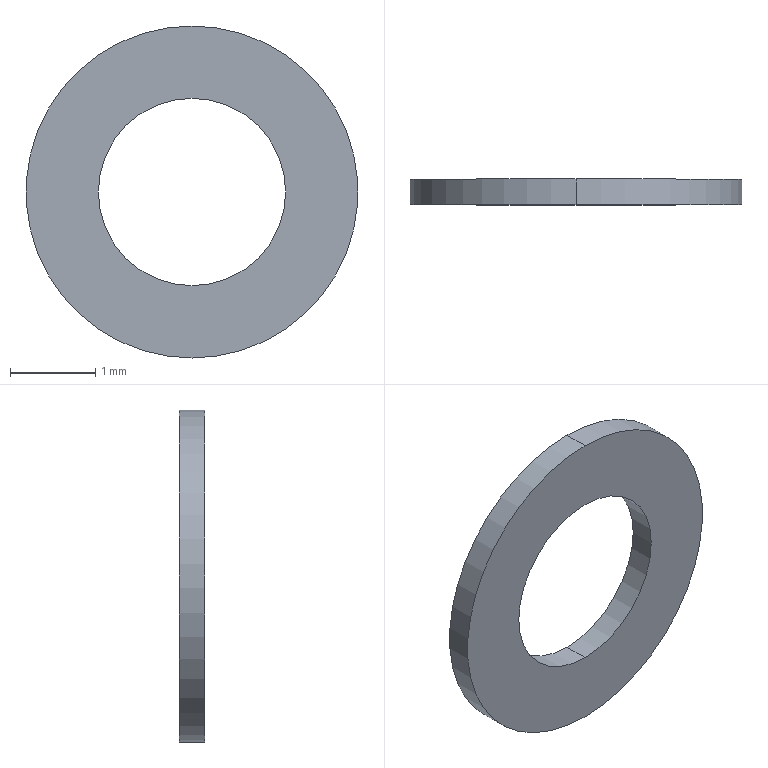Part | STEP file | _1-SO-126050001_1_1_1 | 1 solid | 6 faces | box 3.9 x 0.3 x 3.9 mm | volume 2.443 mm3 | cylinder 4 | plane 2 | commonest cylinder face diameters 2.2 x2 3.9 x2
STEP:
#1=CARTESIAN_POINT('',(0.,0.,0.));
#2=DIRECTION('',(0.,0.,1.));
#3=DIRECTION('',(1.,0.,0.));
#4=AXIS2_PLACEMENT_3D('',#1,#2,#3);
#5=CARTESIAN_POINT('',(-1.5,40.6,-81.15));
#6=VERTEX_POINT('',#5);
#7=CARTESIAN_POINT('',(-1.5,40.9,-81.15));
#8=VERTEX_POINT('',#7);
#9=CARTESIAN_POINT('',(-1.5,40.6,-81.15));
#10=DIRECTION('',(0.,1.,0.));
#11=VECTOR('',#10,1.);
#12=LINE('',#9,#11);
#13=CARTESIAN_POINT('',(-1.5,40.6,-82.25));
#14=DIRECTION('',(0.,1.,0.));
#15=DIRECTION('',(0.,0.,1.));
#16=AXIS2_PLACEMENT_3D('',#13,#14,#15);
#17=CYLINDRICAL_SURFACE('',#16,1.1);
#18=CARTESIAN_POINT('',(6.283,0.));
#19=DIRECTION('',(0.,1.));
#20=VECTOR('',#19,1.);
#21=LINE('',#18,#20);
#22=(GEOMETRIC_REPRESENTATION_CONTEXT(2)PARAMETRIC_REPRESENTATION_CONTEXT()REPRESENTATION_CONTEXT('',''));
#23=DEFINITIONAL_REPRESENTATION('',(#21),#22);
#24=PCURVE('',#17,#23);
#25=CARTESIAN_POINT('',(-1.5,40.6,-82.25));
#26=DIRECTION('',(0.,1.,0.));
#27=DIRECTION('',(0.,0.,1.));
#28=AXIS2_PLACEMENT_3D('',#25,#26,#27);
#29=CYLINDRICAL_SURFACE('',#28,1.1);
#30=CARTESIAN_POINT('',(0.,0.));
#31=DIRECTION('',(0.,1.));
#32=VECTOR('',#31,1.);
#33=LINE('',#30,#32);
#34=(GEOMETRIC_REPRESENTATION_CONTEXT(2)PARAMETRIC_REPRESENTATION_CONTEXT()REPRESENTATION_CONTEXT('',''));
#35=DEFINITIONAL_REPRESENTATION('',(#33),#34);
#36=PCURVE('',#29,#35);
#37=SURFACE_CURVE('',#12,(#24,#36),.PCURVE_S1.);
#38=EDGE_CURVE('',#6,#8,#37,.T.);
#39=ORIENTED_EDGE('',*,*,#38,.T.);
#40=CARTESIAN_POINT('',(-1.5,40.9,-83.35));
#41=VERTEX_POINT('',#40);
#42=CARTESIAN_POINT('',(-1.5,40.9,-82.25));
#43=DIRECTION('',(0.,-1.,0.));
#44=DIRECTION('',(0.,0.,1.));
#45=AXIS2_PLACEMENT_3D('',#42,#43,#44);
#46=CIRCLE('',#45,1.1);
#47=CARTESIAN_POINT('',(6.283,0.3));
#48=DIRECTION('',(-1.,0.));
#49=VECTOR('',#48,1.);
#50=LINE('',#47,#49);
#51=(GEOMETRIC_REPRESENTATION_CONTEXT(2)PARAMETRIC_REPRESENTATION_CONTEXT()REPRESENTATION_CONTEXT('',''));
#52=DEFINITIONAL_REPRESENTATION('',(#50),#51);
#53=PCURVE('',#17,#52);
#54=CARTESIAN_POINT('',(-1.5,40.9,-82.25));
#55=DIRECTION('',(0.,1.,0.));
#56=DIRECTION('',(0.,0.,1.));
#57=AXIS2_PLACEMENT_3D('',#54,#55,#56);
#58=PLANE('',#57);
#59=CARTESIAN_POINT('',(1.1,0.));
#60=CARTESIAN_POINT('',(1.1,-1.905));
#61=CARTESIAN_POINT('',(-0.55,-0.9526));
#62=CARTESIAN_POINT('',(-2.2,0.));
#63=CARTESIAN_POINT('',(-0.55,0.9526));
#64=CARTESIAN_POINT('',(1.1,1.905));
#65=CARTESIAN_POINT('',(1.1,0.));
#66=(BOUNDED_CURVE()B_SPLINE_CURVE(2,(#59,#60,#61,#62,#63,#64,#65),.UNSPECIFIED.,.T.,.F.)B_SPLINE_CURVE_WITH_KNOTS((1,2,2,2,2,1),(-2.094,0.,2.094,4.189,6.283,8.378),.UNSPECIFIED.)CURVE()GEOMETRIC_REPRESENTATION_ITEM()RATIONAL_B_SPLINE_CURVE((1.,0.5,1.,0.5,1.,0.5,1.))REPRESENTATION_ITEM(''));
#67=(GEOMETRIC_REPRESENTATION_CONTEXT(2)PARAMETRIC_REPRESENTATION_CONTEXT()REPRESENTATION_CONTEXT('',''));
#68=DEFINITIONAL_REPRESENTATION('',(#66),#67);
#69=PCURVE('',#58,#68);
#70=SURFACE_CURVE('',#46,(#53,#69),.PCURVE_S1.);
#71=EDGE_CURVE('',#8,#41,#70,.T.);
#72=ORIENTED_EDGE('',*,*,#71,.T.);
#73=CARTESIAN_POINT('',(-1.5,40.6,-83.35));
#74=VERTEX_POINT('',#73);
#75=CARTESIAN_POINT('',(-1.5,40.6,-83.35));
#76=DIRECTION('',(0.,1.,0.));
#77=VECTOR('',#76,1.);
#78=LINE('',#75,#77);
#79=CARTESIAN_POINT('',(3.142,0.));
#80=DIRECTION('',(0.,1.));
#81=VECTOR('',#80,1.);
#82=LINE('',#79,#81);
#83=(GEOMETRIC_REPRESENTATION_CONTEXT(2)PARAMETRIC_REPRESENTATION_CONTEXT()REPRESENTATION_CONTEXT('',''));
#84=DEFINITIONAL_REPRESENTATION('',(#82),#83);
#85=PCURVE('',#17,#84);
#86=CARTESIAN_POINT('',(3.142,0.));
#87=DIRECTION('',(0.,1.));
#88=VECTOR('',#87,1.);
#89=LINE('',#86,#88);
#90=(GEOMETRIC_REPRESENTATION_CONTEXT(2)PARAMETRIC_REPRESENTATION_CONTEXT()REPRESENTATION_CONTEXT('',''));
#91=DEFINITIONAL_REPRESENTATION('',(#89),#90);
#92=PCURVE('',#29,#91);
#93=SURFACE_CURVE('',#78,(#85,#92),.PCURVE_S1.);
#94=EDGE_CURVE('',#74,#41,#93,.T.);
#95=ORIENTED_EDGE('',*,*,#94,.F.);
#96=CARTESIAN_POINT('',(-1.5,40.6,-82.25));
#97=DIRECTION('',(0.,1.,0.));
#98=DIRECTION('',(0.,0.,1.));
#99=AXIS2_PLACEMENT_3D('',#96,#97,#98);
#100=CIRCLE('',#99,1.1);
#101=CARTESIAN_POINT('',(0.,0.));
#102=DIRECTION('',(1.,0.));
#103=VECTOR('',#102,1.);
#104=LINE('',#101,#103);
#105=(GEOMETRIC_REPRESENTATION_CONTEXT(2)PARAMETRIC_REPRESENTATION_CONTEXT()REPRESENTATION_CONTEXT('',''));
#106=DEFINITIONAL_REPRESENTATION('',(#104),#105);
#107=PCURVE('',#17,#106);
#108=CARTESIAN_POINT('',(-1.5,40.6,-82.25));
#109=DIRECTION('',(0.,1.,0.));
#110=DIRECTION('',(0.,0.,1.));
#111=AXIS2_PLACEMENT_3D('',#108,#109,#110);
#112=PLANE('',#111);
#113=CARTESIAN_POINT('',(0.,0.));
#114=DIRECTION('',(1.,0.));
#115=AXIS2_PLACEMENT_2D('',#113,#114);
#116=CIRCLE('',#115,1.1);
#117=(GEOMETRIC_REPRESENTATION_CONTEXT(2)PARAMETRIC_REPRESENTATION_CONTEXT()REPRESENTATION_CONTEXT('',''));
#118=DEFINITIONAL_REPRESENTATION('',(#116),#117);
#119=PCURVE('',#112,#118);
#120=SURFACE_CURVE('',#100,(#107,#119),.PCURVE_S1.);
#121=EDGE_CURVE('',#74,#6,#120,.T.);
#122=ORIENTED_EDGE('',*,*,#121,.T.);
#123=EDGE_LOOP('',(#39,#72,#95,#122));
#124=FACE_BOUND('',#123,.F.);
#125=ADVANCED_FACE('',(#124),#17,.F.);
#126=CARTESIAN_POINT('',(-1.5,40.6,-80.3));
#127=VERTEX_POINT('',#126);
#128=CARTESIAN_POINT('',(-1.5,40.6,-84.2));
#129=VERTEX_POINT('',#128);
#130=CARTESIAN_POINT('',(-1.5,40.6,-82.25));
#131=DIRECTION('',(0.,1.,0.));
#132=DIRECTION('',(0.,0.,1.));
#133=AXIS2_PLACEMENT_3D('',#130,#131,#132);
#134=CIRCLE('',#133,1.95);
#135=CARTESIAN_POINT('',(-1.5,40.6,-82.25));
#136=DIRECTION('',(0.,1.,0.));
#137=DIRECTION('',(0.,0.,1.));
#138=AXIS2_PLACEMENT_3D('',#135,#136,#137);
#139=CYLINDRICAL_SURFACE('',#138,1.95);
#140=CARTESIAN_POINT('',(0.,0.));
#141=DIRECTION('',(1.,0.));
#142=VECTOR('',#141,1.);
#143=LINE('',#140,#142);
#144=(GEOMETRIC_REPRESENTATION_CONTEXT(2)PARAMETRIC_REPRESENTATION_CONTEXT()REPRESENTATION_CONTEXT('',''));
#145=DEFINITIONAL_REPRESENTATION('',(#143),#144);
#146=PCURVE('',#139,#145);
#147=CARTESIAN_POINT('',(0.,0.));
#148=DIRECTION('',(1.,0.));
#149=AXIS2_PLACEMENT_2D('',#147,#148);
#150=CIRCLE('',#149,1.95);
#151=(GEOMETRIC_REPRESENTATION_CONTEXT(2)PARAMETRIC_REPRESENTATION_CONTEXT()REPRESENTATION_CONTEXT('',''));
#152=DEFINITIONAL_REPRESENTATION('',(#150),#151);
#153=PCURVE('',#112,#152);
#154=SURFACE_CURVE('',#134,(#146,#153),.PCURVE_S1.);
#155=EDGE_CURVE('',#127,#129,#154,.T.);
#156=ORIENTED_EDGE('',*,*,#155,.T.);
#157=CARTESIAN_POINT('',(-1.5,40.9,-84.2));
#158=VERTEX_POINT('',#157);
#159=CARTESIAN_POINT('',(-1.5,40.6,-84.2));
#160=DIRECTION('',(0.,1.,0.));
#161=VECTOR('',#160,1.);
#162=LINE('',#159,#161);
#163=CARTESIAN_POINT('',(3.142,0.));
#164=DIRECTION('',(0.,1.));
#165=VECTOR('',#164,1.);
#166=LINE('',#163,#165);
#167=(GEOMETRIC_REPRESENTATION_CONTEXT(2)PARAMETRIC_REPRESENTATION_CONTEXT()REPRESENTATION_CONTEXT('',''));
#168=DEFINITIONAL_REPRESENTATION('',(#166),#167);
#169=PCURVE('',#139,#168);
#170=CARTESIAN_POINT('',(-1.5,40.6,-82.25));
#171=DIRECTION('',(0.,1.,0.));
#172=DIRECTION('',(0.,0.,1.));
#173=AXIS2_PLACEMENT_3D('',#170,#171,#172);
#174=CYLINDRICAL_SURFACE('',#173,1.95);
#175=CARTESIAN_POINT('',(3.142,0.));
#176=DIRECTION('',(0.,1.));
#177=VECTOR('',#176,1.);
#178=LINE('',#175,#177);
#179=(GEOMETRIC_REPRESENTATION_CONTEXT(2)PARAMETRIC_REPRESENTATION_CONTEXT()REPRESENTATION_CONTEXT('',''));
#180=DEFINITIONAL_REPRESENTATION('',(#178),#179);
#181=PCURVE('',#174,#180);
#182=SURFACE_CURVE('',#162,(#169,#181),.PCURVE_S1.);
#183=EDGE_CURVE('',#129,#158,#182,.T.);
#184=ORIENTED_EDGE('',*,*,#183,.T.);
#185=CARTESIAN_POINT('',(-1.5,40.9,-80.3));
#186=VERTEX_POINT('',#185);
#187=CARTESIAN_POINT('',(-1.5,40.9,-82.25));
#188=DIRECTION('',(0.,1.,0.));
#189=DIRECTION('',(0.,0.,1.));
#190=AXIS2_PLACEMENT_3D('',#187,#188,#189);
#191=CIRCLE('',#190,1.95);
#192=CARTESIAN_POINT('',(0.,0.3));
#193=DIRECTION('',(1.,0.));
#194=VECTOR('',#193,1.);
#195=LINE('',#192,#194);
#196=(GEOMETRIC_REPRESENTATION_CONTEXT(2)PARAMETRIC_REPRESENTATION_CONTEXT()REPRESENTATION_CONTEXT('',''));
#197=DEFINITIONAL_REPRESENTATION('',(#195),#196);
#198=PCURVE('',#139,#197);
#199=CARTESIAN_POINT('',(0.,0.));
#200=DIRECTION('',(1.,0.));
#201=AXIS2_PLACEMENT_2D('',#199,#200);
#202=CIRCLE('',#201,1.95);
#203=(GEOMETRIC_REPRESENTATION_CONTEXT(2)PARAMETRIC_REPRESENTATION_CONTEXT()REPRESENTATION_CONTEXT('',''));
#204=DEFINITIONAL_REPRESENTATION('',(#202),#203);
#205=PCURVE('',#58,#204);
#206=SURFACE_CURVE('',#191,(#198,#205),.PCURVE_S1.);
#207=EDGE_CURVE('',#186,#158,#206,.T.);
#208=ORIENTED_EDGE('',*,*,#207,.F.);
#209=CARTESIAN_POINT('',(-1.5,40.6,-80.3));
#210=DIRECTION('',(0.,1.,0.));
#211=VECTOR('',#210,1.);
#212=LINE('',#209,#211);
#213=CARTESIAN_POINT('',(0.,0.));
#214=DIRECTION('',(0.,1.));
#215=VECTOR('',#214,1.);
#216=LINE('',#213,#215);
#217=(GEOMETRIC_REPRESENTATION_CONTEXT(2)PARAMETRIC_REPRESENTATION_CONTEXT()REPRESENTATION_CONTEXT('',''));
#218=DEFINITIONAL_REPRESENTATION('',(#216),#217);
#219=PCURVE('',#139,#218);
#220=CARTESIAN_POINT('',(6.283,0.));
#221=DIRECTION('',(0.,1.));
#222=VECTOR('',#221,1.);
#223=LINE('',#220,#222);
#224=(GEOMETRIC_REPRESENTATION_CONTEXT(2)PARAMETRIC_REPRESENTATION_CONTEXT()REPRESENTATION_CONTEXT('',''));
#225=DEFINITIONAL_REPRESENTATION('',(#223),#224);
#226=PCURVE('',#174,#225);
#227=SURFACE_CURVE('',#212,(#219,#226),.PCURVE_S1.);
#228=EDGE_CURVE('',#127,#186,#227,.T.);
#229=ORIENTED_EDGE('',*,*,#228,.F.);
#230=EDGE_LOOP('',(#156,#184,#208,#229));
#231=FACE_BOUND('',#230,.T.);
#232=ADVANCED_FACE('',(#231),#139,.T.);
#233=ORIENTED_EDGE('',*,*,#71,.T.);
#234=CARTESIAN_POINT('',(-1.5,40.9,-82.25));
#235=DIRECTION('',(0.,-1.,0.));
#236=DIRECTION('',(0.,0.,1.));
#237=AXIS2_PLACEMENT_3D('',#234,#235,#236);
#238=CIRCLE('',#237,1.1);
#239=CARTESIAN_POINT('',(1.1,0.));
#240=CARTESIAN_POINT('',(1.1,-1.905));
#241=CARTESIAN_POINT('',(-0.55,-0.9526));
#242=CARTESIAN_POINT('',(-2.2,0.));
#243=CARTESIAN_POINT('',(-0.55,0.9526));
#244=CARTESIAN_POINT('',(1.1,1.905));
#245=CARTESIAN_POINT('',(1.1,0.));
#246=(BOUNDED_CURVE()B_SPLINE_CURVE(2,(#239,#240,#241,#242,#243,#244,#245),.UNSPECIFIED.,.T.,.F.)B_SPLINE_CURVE_WITH_KNOTS((1,2,2,2,2,1),(-2.094,0.,2.094,4.189,6.283,8.378),.UNSPECIFIED.)CURVE()GEOMETRIC_REPRESENTATION_ITEM()RATIONAL_B_SPLINE_CURVE((1.,0.5,1.,0.5,1.,0.5,1.))REPRESENTATION_ITEM(''));
#247=(GEOMETRIC_REPRESENTATION_CONTEXT(2)PARAMETRIC_REPRESENTATION_CONTEXT()REPRESENTATION_CONTEXT('',''));
#248=DEFINITIONAL_REPRESENTATION('',(#246),#247);
#249=PCURVE('',#58,#248);
#250=CARTESIAN_POINT('',(6.283,0.3));
#251=DIRECTION('',(-1.,0.));
#252=VECTOR('',#251,1.);
#253=LINE('',#250,#252);
#254=(GEOMETRIC_REPRESENTATION_CONTEXT(2)PARAMETRIC_REPRESENTATION_CONTEXT()REPRESENTATION_CONTEXT('',''));
#255=DEFINITIONAL_REPRESENTATION('',(#253),#254);
#256=PCURVE('',#29,#255);
#257=SURFACE_CURVE('',#238,(#249,#256),.PCURVE_S1.);
#258=EDGE_CURVE('',#41,#8,#257,.T.);
#259=ORIENTED_EDGE('',*,*,#258,.T.);
#260=EDGE_LOOP('',(#233,#259));
#261=FACE_BOUND('',#260,.T.);
#262=ORIENTED_EDGE('',*,*,#207,.T.);
#263=CARTESIAN_POINT('',(-1.5,40.9,-82.25));
#264=DIRECTION('',(0.,1.,0.));
#265=DIRECTION('',(0.,0.,1.));
#266=AXIS2_PLACEMENT_3D('',#263,#264,#265);
#267=CIRCLE('',#266,1.95);
#268=CARTESIAN_POINT('',(0.,0.));
#269=DIRECTION('',(1.,0.));
#270=AXIS2_PLACEMENT_2D('',#268,#269);
#271=CIRCLE('',#270,1.95);
#272=(GEOMETRIC_REPRESENTATION_CONTEXT(2)PARAMETRIC_REPRESENTATION_CONTEXT()REPRESENTATION_CONTEXT('',''));
#273=DEFINITIONAL_REPRESENTATION('',(#271),#272);
#274=PCURVE('',#58,#273);
#275=CARTESIAN_POINT('',(0.,0.3));
#276=DIRECTION('',(1.,0.));
#277=VECTOR('',#276,1.);
#278=LINE('',#275,#277);
#279=(GEOMETRIC_REPRESENTATION_CONTEXT(2)PARAMETRIC_REPRESENTATION_CONTEXT()REPRESENTATION_CONTEXT('',''));
#280=DEFINITIONAL_REPRESENTATION('',(#278),#279);
#281=PCURVE('',#174,#280);
#282=SURFACE_CURVE('',#267,(#274,#281),.PCURVE_S1.);
#283=EDGE_CURVE('',#158,#186,#282,.T.);
#284=ORIENTED_EDGE('',*,*,#283,.T.);
#285=EDGE_LOOP('',(#262,#284));
#286=FACE_BOUND('',#285,.T.);
#287=ADVANCED_FACE('',(#261,#286),#58,.T.);
#288=ORIENTED_EDGE('',*,*,#258,.T.);
#289=ORIENTED_EDGE('',*,*,#38,.F.);
#290=CARTESIAN_POINT('',(-1.5,40.6,-82.25));
#291=DIRECTION('',(0.,1.,0.));
#292=DIRECTION('',(0.,0.,1.));
#293=AXIS2_PLACEMENT_3D('',#290,#291,#292);
#294=CIRCLE('',#293,1.1);
#295=CARTESIAN_POINT('',(0.,0.));
#296=DIRECTION('',(1.,0.));
#297=VECTOR('',#296,1.);
#298=LINE('',#295,#297);
#299=(GEOMETRIC_REPRESENTATION_CONTEXT(2)PARAMETRIC_REPRESENTATION_CONTEXT()REPRESENTATION_CONTEXT('',''));
#300=DEFINITIONAL_REPRESENTATION('',(#298),#299);
#301=PCURVE('',#29,#300);
#302=CARTESIAN_POINT('',(0.,0.));
#303=DIRECTION('',(1.,0.));
#304=AXIS2_PLACEMENT_2D('',#302,#303);
#305=CIRCLE('',#304,1.1);
#306=(GEOMETRIC_REPRESENTATION_CONTEXT(2)PARAMETRIC_REPRESENTATION_CONTEXT()REPRESENTATION_CONTEXT('',''));
#307=DEFINITIONAL_REPRESENTATION('',(#305),#306);
#308=PCURVE('',#112,#307);
#309=SURFACE_CURVE('',#294,(#301,#308),.PCURVE_S1.);
#310=EDGE_CURVE('',#6,#74,#309,.T.);
#311=ORIENTED_EDGE('',*,*,#310,.T.);
#312=ORIENTED_EDGE('',*,*,#94,.T.);
#313=EDGE_LOOP('',(#288,#289,#311,#312));
#314=FACE_BOUND('',#313,.F.);
#315=ADVANCED_FACE('',(#314),#29,.F.);
#316=ORIENTED_EDGE('',*,*,#183,.F.);
#317=CARTESIAN_POINT('',(-1.5,40.6,-82.25));
#318=DIRECTION('',(0.,1.,0.));
#319=DIRECTION('',(0.,0.,1.));
#320=AXIS2_PLACEMENT_3D('',#317,#318,#319);
#321=CIRCLE('',#320,1.95);
#322=CARTESIAN_POINT('',(0.,0.));
#323=DIRECTION('',(1.,0.));
#324=VECTOR('',#323,1.);
#325=LINE('',#322,#324);
#326=(GEOMETRIC_REPRESENTATION_CONTEXT(2)PARAMETRIC_REPRESENTATION_CONTEXT()REPRESENTATION_CONTEXT('',''));
#327=DEFINITIONAL_REPRESENTATION('',(#325),#326);
#328=PCURVE('',#174,#327);
#329=CARTESIAN_POINT('',(0.,0.));
#330=DIRECTION('',(1.,0.));
#331=AXIS2_PLACEMENT_2D('',#329,#330);
#332=CIRCLE('',#331,1.95);
#333=(GEOMETRIC_REPRESENTATION_CONTEXT(2)PARAMETRIC_REPRESENTATION_CONTEXT()REPRESENTATION_CONTEXT('',''));
#334=DEFINITIONAL_REPRESENTATION('',(#332),#333);
#335=PCURVE('',#112,#334);
#336=SURFACE_CURVE('',#321,(#328,#335),.PCURVE_S1.);
#337=EDGE_CURVE('',#129,#127,#336,.T.);
#338=ORIENTED_EDGE('',*,*,#337,.T.);
#339=ORIENTED_EDGE('',*,*,#228,.T.);
#340=ORIENTED_EDGE('',*,*,#283,.F.);
#341=EDGE_LOOP('',(#316,#338,#339,#340));
#342=FACE_BOUND('',#341,.T.);
#343=ADVANCED_FACE('',(#342),#174,.T.);
#344=ORIENTED_EDGE('',*,*,#310,.T.);
#345=ORIENTED_EDGE('',*,*,#121,.T.);
#346=EDGE_LOOP('',(#344,#345));
#347=FACE_BOUND('',#346,.T.);
#348=ORIENTED_EDGE('',*,*,#155,.F.);
#349=ORIENTED_EDGE('',*,*,#337,.F.);
#350=EDGE_LOOP('',(#348,#349));
#351=FACE_BOUND('',#350,.T.);
#352=ADVANCED_FACE('',(#347,#351),#112,.F.);
#353=CLOSED_SHELL('',(#125,#232,#287,#315,#343,#352));
#354=MANIFOLD_SOLID_BREP('',#353);
#355=(LENGTH_UNIT()NAMED_UNIT(*)SI_UNIT(.MILLI.,.METRE.));
#356=UNCERTAINTY_MEASURE_WITH_UNIT(LENGTH_MEASURE(0.0000001),#355,'','');
#357=(NAMED_UNIT(*)PLANE_ANGLE_UNIT()SI_UNIT($,.RADIAN.));
#358=(NAMED_UNIT(*)SI_UNIT($,.STERADIAN.)SOLID_ANGLE_UNIT());
#359=(GEOMETRIC_REPRESENTATION_CONTEXT(3)GLOBAL_UNCERTAINTY_ASSIGNED_CONTEXT((#356))GLOBAL_UNIT_ASSIGNED_CONTEXT((#355,#357,#358))REPRESENTATION_CONTEXT('',''));
#360=ADVANCED_BREP_SHAPE_REPRESENTATION('',(#4,#354),#359);